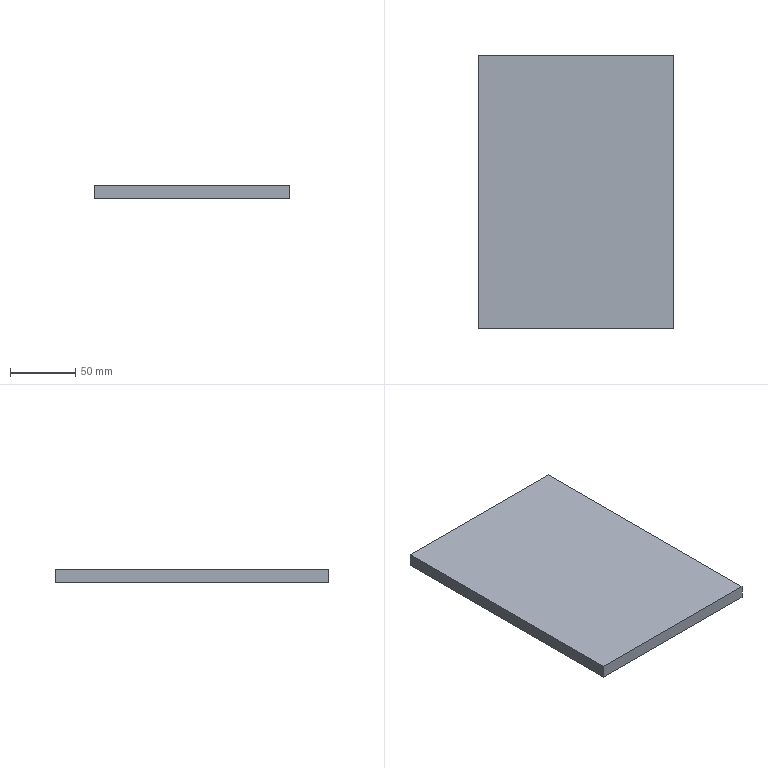Part | STEP file | PN_0009 support base plate 150x210_Default<As Machined> | 1 solid | 6 faces | box 150 x 210 x 10 mm | volume 315000 mm3 | plane 6
STEP:
#1=CARTESIAN_POINT('',(0.,0.,0.));
#2=DIRECTION('',(0.,0.,1.));
#3=DIRECTION('',(1.,0.,0.));
#4=AXIS2_PLACEMENT_3D('',#1,#2,#3);
#5=CARTESIAN_POINT('',(75.,-105.,0.));
#6=VERTEX_POINT('',#5);
#7=CARTESIAN_POINT('',(75.,105.,0.));
#8=VERTEX_POINT('',#7);
#9=CARTESIAN_POINT('',(75.,105.,0.));
#10=DIRECTION('',(0.,1.,0.));
#11=VECTOR('',#10,1.);
#12=LINE('',#9,#11);
#13=CARTESIAN_POINT('',(75.,105.,10.));
#14=DIRECTION('',(-1.,0.,0.));
#15=DIRECTION('',(0.,0.,1.));
#16=AXIS2_PLACEMENT_3D('',#13,#14,#15);
#17=PLANE('',#16);
#18=CARTESIAN_POINT('',(-10.,0.));
#19=DIRECTION('',(0.,1.));
#20=VECTOR('',#19,1.);
#21=LINE('',#18,#20);
#22=(GEOMETRIC_REPRESENTATION_CONTEXT(2)PARAMETRIC_REPRESENTATION_CONTEXT()REPRESENTATION_CONTEXT('',''));
#23=DEFINITIONAL_REPRESENTATION('',(#21),#22);
#24=PCURVE('',#17,#23);
#25=CARTESIAN_POINT('',(0.,0.,0.));
#26=DIRECTION('',(0.,0.,1.));
#27=DIRECTION('',(1.,0.,0.));
#28=AXIS2_PLACEMENT_3D('',#25,#26,#27);
#29=PLANE('',#28);
#30=CARTESIAN_POINT('',(75.,105.));
#31=DIRECTION('',(0.,1.));
#32=VECTOR('',#31,1.);
#33=LINE('',#30,#32);
#34=(GEOMETRIC_REPRESENTATION_CONTEXT(2)PARAMETRIC_REPRESENTATION_CONTEXT()REPRESENTATION_CONTEXT('',''));
#35=DEFINITIONAL_REPRESENTATION('',(#33),#34);
#36=PCURVE('',#29,#35);
#37=SURFACE_CURVE('',#12,(#24,#36),.PCURVE_S1.);
#38=EDGE_CURVE('',#6,#8,#37,.T.);
#39=ORIENTED_EDGE('',*,*,#38,.T.);
#40=CARTESIAN_POINT('',(75.,105.,10.));
#41=VERTEX_POINT('',#40);
#42=CARTESIAN_POINT('',(75.,105.,10.));
#43=DIRECTION('',(0.,0.,-1.));
#44=VECTOR('',#43,1.);
#45=LINE('',#42,#44);
#46=CARTESIAN_POINT('',(0.,0.));
#47=DIRECTION('',(-1.,0.));
#48=VECTOR('',#47,1.);
#49=LINE('',#46,#48);
#50=(GEOMETRIC_REPRESENTATION_CONTEXT(2)PARAMETRIC_REPRESENTATION_CONTEXT()REPRESENTATION_CONTEXT('',''));
#51=DEFINITIONAL_REPRESENTATION('',(#49),#50);
#52=PCURVE('',#17,#51);
#53=CARTESIAN_POINT('',(-75.,105.,10.));
#54=DIRECTION('',(0.,-1.,0.));
#55=DIRECTION('',(0.,0.,-1.));
#56=AXIS2_PLACEMENT_3D('',#53,#54,#55);
#57=PLANE('',#56);
#58=CARTESIAN_POINT('',(0.,150.));
#59=DIRECTION('',(1.,0.));
#60=VECTOR('',#59,1.);
#61=LINE('',#58,#60);
#62=(GEOMETRIC_REPRESENTATION_CONTEXT(2)PARAMETRIC_REPRESENTATION_CONTEXT()REPRESENTATION_CONTEXT('',''));
#63=DEFINITIONAL_REPRESENTATION('',(#61),#62);
#64=PCURVE('',#57,#63);
#65=SURFACE_CURVE('',#45,(#52,#64),.PCURVE_S1.);
#66=EDGE_CURVE('',#41,#8,#65,.T.);
#67=ORIENTED_EDGE('',*,*,#66,.F.);
#68=CARTESIAN_POINT('',(75.,-105.,10.));
#69=VERTEX_POINT('',#68);
#70=CARTESIAN_POINT('',(75.,105.,10.));
#71=DIRECTION('',(0.,1.,0.));
#72=VECTOR('',#71,1.);
#73=LINE('',#70,#72);
#74=CARTESIAN_POINT('',(0.,0.));
#75=DIRECTION('',(0.,1.));
#76=VECTOR('',#75,1.);
#77=LINE('',#74,#76);
#78=(GEOMETRIC_REPRESENTATION_CONTEXT(2)PARAMETRIC_REPRESENTATION_CONTEXT()REPRESENTATION_CONTEXT('',''));
#79=DEFINITIONAL_REPRESENTATION('',(#77),#78);
#80=PCURVE('',#17,#79);
#81=CARTESIAN_POINT('',(0.,0.,10.));
#82=DIRECTION('',(0.,0.,1.));
#83=DIRECTION('',(1.,0.,0.));
#84=AXIS2_PLACEMENT_3D('',#81,#82,#83);
#85=PLANE('',#84);
#86=CARTESIAN_POINT('',(75.,105.));
#87=DIRECTION('',(0.,1.));
#88=VECTOR('',#87,1.);
#89=LINE('',#86,#88);
#90=(GEOMETRIC_REPRESENTATION_CONTEXT(2)PARAMETRIC_REPRESENTATION_CONTEXT()REPRESENTATION_CONTEXT('',''));
#91=DEFINITIONAL_REPRESENTATION('',(#89),#90);
#92=PCURVE('',#85,#91);
#93=SURFACE_CURVE('',#73,(#80,#92),.PCURVE_S1.);
#94=EDGE_CURVE('',#69,#41,#93,.T.);
#95=ORIENTED_EDGE('',*,*,#94,.F.);
#96=CARTESIAN_POINT('',(75.,-105.,10.));
#97=DIRECTION('',(0.,0.,-1.));
#98=VECTOR('',#97,1.);
#99=LINE('',#96,#98);
#100=CARTESIAN_POINT('',(0.,-210.));
#101=DIRECTION('',(-1.,0.));
#102=VECTOR('',#101,1.);
#103=LINE('',#100,#102);
#104=(GEOMETRIC_REPRESENTATION_CONTEXT(2)PARAMETRIC_REPRESENTATION_CONTEXT()REPRESENTATION_CONTEXT('',''));
#105=DEFINITIONAL_REPRESENTATION('',(#103),#104);
#106=PCURVE('',#17,#105);
#107=CARTESIAN_POINT('',(-75.,-105.,10.));
#108=DIRECTION('',(0.,1.,0.));
#109=DIRECTION('',(0.,0.,1.));
#110=AXIS2_PLACEMENT_3D('',#107,#108,#109);
#111=PLANE('',#110);
#112=CARTESIAN_POINT('',(0.,150.));
#113=DIRECTION('',(-1.,0.));
#114=VECTOR('',#113,1.);
#115=LINE('',#112,#114);
#116=(GEOMETRIC_REPRESENTATION_CONTEXT(2)PARAMETRIC_REPRESENTATION_CONTEXT()REPRESENTATION_CONTEXT('',''));
#117=DEFINITIONAL_REPRESENTATION('',(#115),#116);
#118=PCURVE('',#111,#117);
#119=SURFACE_CURVE('',#99,(#106,#118),.PCURVE_S1.);
#120=EDGE_CURVE('',#69,#6,#119,.T.);
#121=ORIENTED_EDGE('',*,*,#120,.T.);
#122=EDGE_LOOP('',(#39,#67,#95,#121));
#123=FACE_BOUND('',#122,.T.);
#124=ADVANCED_FACE('',(#123),#17,.F.);
#125=CARTESIAN_POINT('',(-75.,105.,0.));
#126=VERTEX_POINT('',#125);
#127=CARTESIAN_POINT('',(-75.,105.,0.));
#128=DIRECTION('',(-1.,0.,0.));
#129=VECTOR('',#128,1.);
#130=LINE('',#127,#129);
#131=CARTESIAN_POINT('',(10.,0.));
#132=DIRECTION('',(0.,-1.));
#133=VECTOR('',#132,1.);
#134=LINE('',#131,#133);
#135=(GEOMETRIC_REPRESENTATION_CONTEXT(2)PARAMETRIC_REPRESENTATION_CONTEXT()REPRESENTATION_CONTEXT('',''));
#136=DEFINITIONAL_REPRESENTATION('',(#134),#135);
#137=PCURVE('',#57,#136);
#138=CARTESIAN_POINT('',(-75.,105.));
#139=DIRECTION('',(-1.,0.));
#140=VECTOR('',#139,1.);
#141=LINE('',#138,#140);
#142=(GEOMETRIC_REPRESENTATION_CONTEXT(2)PARAMETRIC_REPRESENTATION_CONTEXT()REPRESENTATION_CONTEXT('',''));
#143=DEFINITIONAL_REPRESENTATION('',(#141),#142);
#144=PCURVE('',#29,#143);
#145=SURFACE_CURVE('',#130,(#137,#144),.PCURVE_S1.);
#146=EDGE_CURVE('',#8,#126,#145,.T.);
#147=ORIENTED_EDGE('',*,*,#146,.T.);
#148=CARTESIAN_POINT('',(-75.,105.,10.));
#149=VERTEX_POINT('',#148);
#150=CARTESIAN_POINT('',(-75.,105.,10.));
#151=DIRECTION('',(0.,0.,-1.));
#152=VECTOR('',#151,1.);
#153=LINE('',#150,#152);
#154=CARTESIAN_POINT('',(0.,0.));
#155=DIRECTION('',(1.,0.));
#156=VECTOR('',#155,1.);
#157=LINE('',#154,#156);
#158=(GEOMETRIC_REPRESENTATION_CONTEXT(2)PARAMETRIC_REPRESENTATION_CONTEXT()REPRESENTATION_CONTEXT('',''));
#159=DEFINITIONAL_REPRESENTATION('',(#157),#158);
#160=PCURVE('',#57,#159);
#161=CARTESIAN_POINT('',(-75.,105.,10.));
#162=DIRECTION('',(1.,0.,0.));
#163=DIRECTION('',(0.,0.,-1.));
#164=AXIS2_PLACEMENT_3D('',#161,#162,#163);
#165=PLANE('',#164);
#166=CARTESIAN_POINT('',(0.,0.));
#167=DIRECTION('',(1.,0.));
#168=VECTOR('',#167,1.);
#169=LINE('',#166,#168);
#170=(GEOMETRIC_REPRESENTATION_CONTEXT(2)PARAMETRIC_REPRESENTATION_CONTEXT()REPRESENTATION_CONTEXT('',''));
#171=DEFINITIONAL_REPRESENTATION('',(#169),#170);
#172=PCURVE('',#165,#171);
#173=SURFACE_CURVE('',#153,(#160,#172),.PCURVE_S1.);
#174=EDGE_CURVE('',#149,#126,#173,.T.);
#175=ORIENTED_EDGE('',*,*,#174,.F.);
#176=CARTESIAN_POINT('',(-75.,105.,10.));
#177=DIRECTION('',(-1.,0.,0.));
#178=VECTOR('',#177,1.);
#179=LINE('',#176,#178);
#180=CARTESIAN_POINT('',(0.,0.));
#181=DIRECTION('',(0.,-1.));
#182=VECTOR('',#181,1.);
#183=LINE('',#180,#182);
#184=(GEOMETRIC_REPRESENTATION_CONTEXT(2)PARAMETRIC_REPRESENTATION_CONTEXT()REPRESENTATION_CONTEXT('',''));
#185=DEFINITIONAL_REPRESENTATION('',(#183),#184);
#186=PCURVE('',#57,#185);
#187=CARTESIAN_POINT('',(-75.,105.));
#188=DIRECTION('',(-1.,0.));
#189=VECTOR('',#188,1.);
#190=LINE('',#187,#189);
#191=(GEOMETRIC_REPRESENTATION_CONTEXT(2)PARAMETRIC_REPRESENTATION_CONTEXT()REPRESENTATION_CONTEXT('',''));
#192=DEFINITIONAL_REPRESENTATION('',(#190),#191);
#193=PCURVE('',#85,#192);
#194=SURFACE_CURVE('',#179,(#186,#193),.PCURVE_S1.);
#195=EDGE_CURVE('',#41,#149,#194,.T.);
#196=ORIENTED_EDGE('',*,*,#195,.F.);
#197=ORIENTED_EDGE('',*,*,#66,.T.);
#198=EDGE_LOOP('',(#147,#175,#196,#197));
#199=FACE_BOUND('',#198,.T.);
#200=ADVANCED_FACE('',(#199),#57,.F.);
#201=CARTESIAN_POINT('',(-75.,-105.,0.));
#202=VERTEX_POINT('',#201);
#203=CARTESIAN_POINT('',(-75.,105.,0.));
#204=DIRECTION('',(0.,-1.,0.));
#205=VECTOR('',#204,1.);
#206=LINE('',#203,#205);
#207=CARTESIAN_POINT('',(10.,0.));
#208=DIRECTION('',(0.,-1.));
#209=VECTOR('',#208,1.);
#210=LINE('',#207,#209);
#211=(GEOMETRIC_REPRESENTATION_CONTEXT(2)PARAMETRIC_REPRESENTATION_CONTEXT()REPRESENTATION_CONTEXT('',''));
#212=DEFINITIONAL_REPRESENTATION('',(#210),#211);
#213=PCURVE('',#165,#212);
#214=CARTESIAN_POINT('',(-75.,105.));
#215=DIRECTION('',(0.,-1.));
#216=VECTOR('',#215,1.);
#217=LINE('',#214,#216);
#218=(GEOMETRIC_REPRESENTATION_CONTEXT(2)PARAMETRIC_REPRESENTATION_CONTEXT()REPRESENTATION_CONTEXT('',''));
#219=DEFINITIONAL_REPRESENTATION('',(#217),#218);
#220=PCURVE('',#29,#219);
#221=SURFACE_CURVE('',#206,(#213,#220),.PCURVE_S1.);
#222=EDGE_CURVE('',#126,#202,#221,.T.);
#223=ORIENTED_EDGE('',*,*,#222,.T.);
#224=CARTESIAN_POINT('',(-75.,-105.,10.));
#225=VERTEX_POINT('',#224);
#226=CARTESIAN_POINT('',(-75.,-105.,10.));
#227=DIRECTION('',(0.,0.,-1.));
#228=VECTOR('',#227,1.);
#229=LINE('',#226,#228);
#230=CARTESIAN_POINT('',(0.,-210.));
#231=DIRECTION('',(1.,0.));
#232=VECTOR('',#231,1.);
#233=LINE('',#230,#232);
#234=(GEOMETRIC_REPRESENTATION_CONTEXT(2)PARAMETRIC_REPRESENTATION_CONTEXT()REPRESENTATION_CONTEXT('',''));
#235=DEFINITIONAL_REPRESENTATION('',(#233),#234);
#236=PCURVE('',#165,#235);
#237=CARTESIAN_POINT('',(0.,0.));
#238=DIRECTION('',(-1.,0.));
#239=VECTOR('',#238,1.);
#240=LINE('',#237,#239);
#241=(GEOMETRIC_REPRESENTATION_CONTEXT(2)PARAMETRIC_REPRESENTATION_CONTEXT()REPRESENTATION_CONTEXT('',''));
#242=DEFINITIONAL_REPRESENTATION('',(#240),#241);
#243=PCURVE('',#111,#242);
#244=SURFACE_CURVE('',#229,(#236,#243),.PCURVE_S1.);
#245=EDGE_CURVE('',#225,#202,#244,.T.);
#246=ORIENTED_EDGE('',*,*,#245,.F.);
#247=CARTESIAN_POINT('',(-75.,105.,10.));
#248=DIRECTION('',(0.,-1.,0.));
#249=VECTOR('',#248,1.);
#250=LINE('',#247,#249);
#251=CARTESIAN_POINT('',(0.,0.));
#252=DIRECTION('',(0.,-1.));
#253=VECTOR('',#252,1.);
#254=LINE('',#251,#253);
#255=(GEOMETRIC_REPRESENTATION_CONTEXT(2)PARAMETRIC_REPRESENTATION_CONTEXT()REPRESENTATION_CONTEXT('',''));
#256=DEFINITIONAL_REPRESENTATION('',(#254),#255);
#257=PCURVE('',#165,#256);
#258=CARTESIAN_POINT('',(-75.,105.));
#259=DIRECTION('',(0.,-1.));
#260=VECTOR('',#259,1.);
#261=LINE('',#258,#260);
#262=(GEOMETRIC_REPRESENTATION_CONTEXT(2)PARAMETRIC_REPRESENTATION_CONTEXT()REPRESENTATION_CONTEXT('',''));
#263=DEFINITIONAL_REPRESENTATION('',(#261),#262);
#264=PCURVE('',#85,#263);
#265=SURFACE_CURVE('',#250,(#257,#264),.PCURVE_S1.);
#266=EDGE_CURVE('',#149,#225,#265,.T.);
#267=ORIENTED_EDGE('',*,*,#266,.F.);
#268=ORIENTED_EDGE('',*,*,#174,.T.);
#269=EDGE_LOOP('',(#223,#246,#267,#268));
#270=FACE_BOUND('',#269,.T.);
#271=ADVANCED_FACE('',(#270),#165,.F.);
#272=CARTESIAN_POINT('',(-75.,-105.,0.));
#273=DIRECTION('',(1.,0.,0.));
#274=VECTOR('',#273,1.);
#275=LINE('',#272,#274);
#276=CARTESIAN_POINT('',(-10.,0.));
#277=DIRECTION('',(0.,1.));
#278=VECTOR('',#277,1.);
#279=LINE('',#276,#278);
#280=(GEOMETRIC_REPRESENTATION_CONTEXT(2)PARAMETRIC_REPRESENTATION_CONTEXT()REPRESENTATION_CONTEXT('',''));
#281=DEFINITIONAL_REPRESENTATION('',(#279),#280);
#282=PCURVE('',#111,#281);
#283=CARTESIAN_POINT('',(-75.,-105.));
#284=DIRECTION('',(1.,0.));
#285=VECTOR('',#284,1.);
#286=LINE('',#283,#285);
#287=(GEOMETRIC_REPRESENTATION_CONTEXT(2)PARAMETRIC_REPRESENTATION_CONTEXT()REPRESENTATION_CONTEXT('',''));
#288=DEFINITIONAL_REPRESENTATION('',(#286),#287);
#289=PCURVE('',#29,#288);
#290=SURFACE_CURVE('',#275,(#282,#289),.PCURVE_S1.);
#291=EDGE_CURVE('',#202,#6,#290,.T.);
#292=ORIENTED_EDGE('',*,*,#291,.T.);
#293=ORIENTED_EDGE('',*,*,#120,.F.);
#294=CARTESIAN_POINT('',(-75.,-105.,10.));
#295=DIRECTION('',(1.,0.,0.));
#296=VECTOR('',#295,1.);
#297=LINE('',#294,#296);
#298=CARTESIAN_POINT('',(0.,0.));
#299=DIRECTION('',(0.,1.));
#300=VECTOR('',#299,1.);
#301=LINE('',#298,#300);
#302=(GEOMETRIC_REPRESENTATION_CONTEXT(2)PARAMETRIC_REPRESENTATION_CONTEXT()REPRESENTATION_CONTEXT('',''));
#303=DEFINITIONAL_REPRESENTATION('',(#301),#302);
#304=PCURVE('',#111,#303);
#305=CARTESIAN_POINT('',(-75.,-105.));
#306=DIRECTION('',(1.,0.));
#307=VECTOR('',#306,1.);
#308=LINE('',#305,#307);
#309=(GEOMETRIC_REPRESENTATION_CONTEXT(2)PARAMETRIC_REPRESENTATION_CONTEXT()REPRESENTATION_CONTEXT('',''));
#310=DEFINITIONAL_REPRESENTATION('',(#308),#309);
#311=PCURVE('',#85,#310);
#312=SURFACE_CURVE('',#297,(#304,#311),.PCURVE_S1.);
#313=EDGE_CURVE('',#225,#69,#312,.T.);
#314=ORIENTED_EDGE('',*,*,#313,.F.);
#315=ORIENTED_EDGE('',*,*,#245,.T.);
#316=EDGE_LOOP('',(#292,#293,#314,#315));
#317=FACE_BOUND('',#316,.T.);
#318=ADVANCED_FACE('',(#317),#111,.F.);
#319=ORIENTED_EDGE('',*,*,#94,.T.);
#320=ORIENTED_EDGE('',*,*,#195,.T.);
#321=ORIENTED_EDGE('',*,*,#266,.T.);
#322=ORIENTED_EDGE('',*,*,#313,.T.);
#323=EDGE_LOOP('',(#319,#320,#321,#322));
#324=FACE_BOUND('',#323,.T.);
#325=ADVANCED_FACE('',(#324),#85,.T.);
#326=ORIENTED_EDGE('',*,*,#38,.F.);
#327=ORIENTED_EDGE('',*,*,#291,.F.);
#328=ORIENTED_EDGE('',*,*,#222,.F.);
#329=ORIENTED_EDGE('',*,*,#146,.F.);
#330=EDGE_LOOP('',(#326,#327,#328,#329));
#331=FACE_BOUND('',#330,.T.);
#332=ADVANCED_FACE('',(#331),#29,.F.);
#333=CLOSED_SHELL('',(#124,#200,#271,#318,#325,#332));
#334=MANIFOLD_SOLID_BREP('',#333);
#335=(LENGTH_UNIT()NAMED_UNIT(*)SI_UNIT(.MILLI.,.METRE.));
#336=UNCERTAINTY_MEASURE_WITH_UNIT(LENGTH_MEASURE(0.0000001),#335,'','');
#337=(NAMED_UNIT(*)PLANE_ANGLE_UNIT()SI_UNIT($,.RADIAN.));
#338=(NAMED_UNIT(*)SI_UNIT($,.STERADIAN.)SOLID_ANGLE_UNIT());
#339=(GEOMETRIC_REPRESENTATION_CONTEXT(3)GLOBAL_UNCERTAINTY_ASSIGNED_CONTEXT((#336))GLOBAL_UNIT_ASSIGNED_CONTEXT((#335,#337,#338))REPRESENTATION_CONTEXT('',''));
#340=ADVANCED_BREP_SHAPE_REPRESENTATION('',(#4,#334),#339);